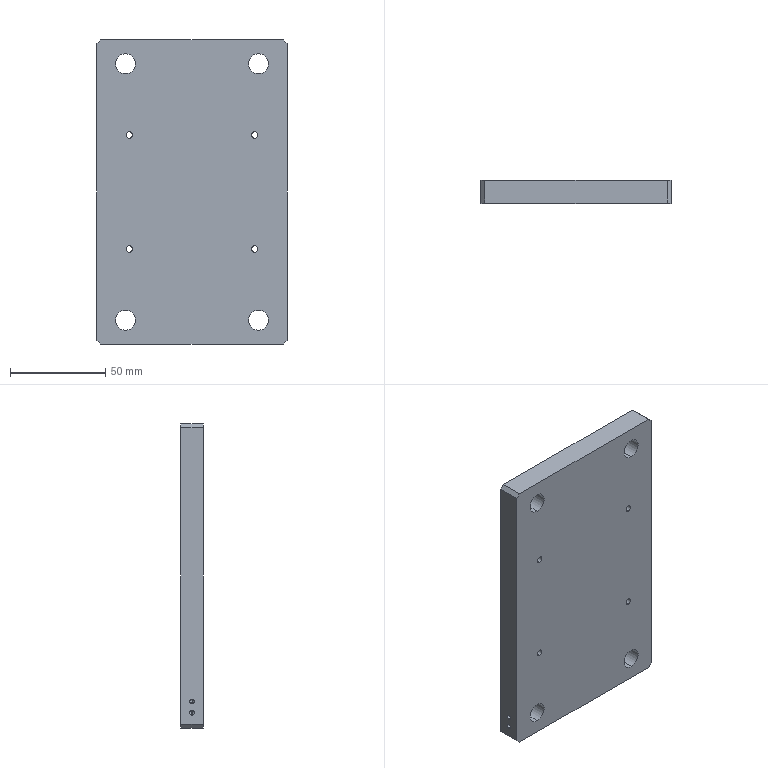Part | STEP file | PN_0009 | 1 solid | 42 faces | box 100 x 12 x 160 mm | volume 187185 mm3 | cylinder 24 | plane 10 | cone 8 | commonest cylinder face diameters 2.5 x8 3.3 x8 10.5 x8